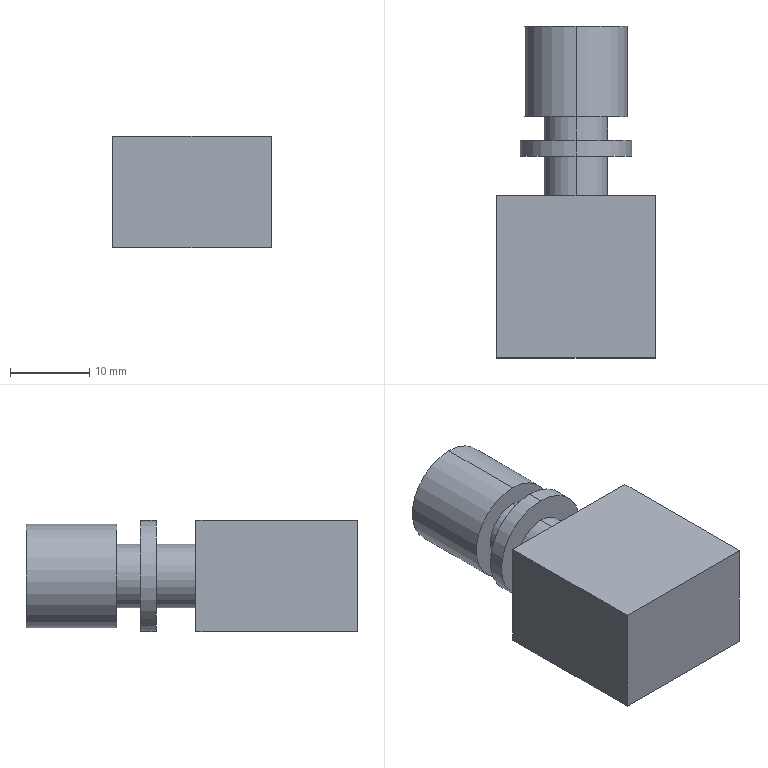Part | STEP file | A2A-4B | 1 solid | 18 faces | box 20 x 41.8 x 14 mm | volume 7935 mm3 | plane 10 | cylinder 8 | commonest cylinder face diameters 8 x4 13 x2 14 x2
STEP:
#1=CARTESIAN_POINT('',(0.,0.,0.));
#2=DIRECTION('',(0.,0.,1.));
#3=DIRECTION('',(1.,0.,0.));
#4=AXIS2_PLACEMENT_3D('',#1,#2,#3);
#5=CARTESIAN_POINT('',(0.,20.4,-4.));
#6=VERTEX_POINT('',#5);
#7=CARTESIAN_POINT('',(0.,20.4,4.));
#8=VERTEX_POINT('',#7);
#9=CARTESIAN_POINT('',(0.,20.4,0.));
#10=DIRECTION('',(0.,-1.,0.));
#11=DIRECTION('',(0.,0.,1.));
#12=AXIS2_PLACEMENT_3D('',#9,#10,#11);
#13=CIRCLE('',#12,4.);
#14=CARTESIAN_POINT('',(0.,41.8,0.));
#15=DIRECTION('',(0.,1.,0.));
#16=DIRECTION('',(0.,0.,1.));
#17=AXIS2_PLACEMENT_3D('',#14,#15,#16);
#18=CYLINDRICAL_SURFACE('',#17,4.);
#19=CARTESIAN_POINT('',(6.283,-21.4));
#20=DIRECTION('',(-1.,0.));
#21=VECTOR('',#20,1.);
#22=LINE('',#19,#21);
#23=(GEOMETRIC_REPRESENTATION_CONTEXT(2)PARAMETRIC_REPRESENTATION_CONTEXT()REPRESENTATION_CONTEXT('',''));
#24=DEFINITIONAL_REPRESENTATION('',(#22),#23);
#25=PCURVE('',#18,#24);
#26=CARTESIAN_POINT('',(10.,20.4,7.));
#27=DIRECTION('',(0.,1.,0.));
#28=DIRECTION('',(0.,0.,1.));
#29=AXIS2_PLACEMENT_3D('',#26,#27,#28);
#30=PLANE('',#29);
#31=CARTESIAN_POINT('',(-3.,-10.));
#32=CARTESIAN_POINT('',(-3.,-16.928));
#33=CARTESIAN_POINT('',(-9.,-13.464));
#34=CARTESIAN_POINT('',(-15.,-10.));
#35=CARTESIAN_POINT('',(-9.,-6.536));
#36=CARTESIAN_POINT('',(-3.,-3.072));
#37=CARTESIAN_POINT('',(-3.,-10.));
#38=(BOUNDED_CURVE()B_SPLINE_CURVE(2,(#31,#32,#33,#34,#35,#36,#37),.UNSPECIFIED.,.T.,.F.)B_SPLINE_CURVE_WITH_KNOTS((1,2,2,2,2,1),(-2.094,0.,2.094,4.189,6.283,8.378),.UNSPECIFIED.)CURVE()GEOMETRIC_REPRESENTATION_ITEM()RATIONAL_B_SPLINE_CURVE((1.,0.5,1.,0.5,1.,0.5,1.))REPRESENTATION_ITEM(''));
#39=(GEOMETRIC_REPRESENTATION_CONTEXT(2)PARAMETRIC_REPRESENTATION_CONTEXT()REPRESENTATION_CONTEXT('',''));
#40=DEFINITIONAL_REPRESENTATION('',(#38),#39);
#41=PCURVE('',#30,#40);
#42=SURFACE_CURVE('',#13,(#25,#41),.PCURVE_S1.);
#43=EDGE_CURVE('',#6,#8,#42,.T.);
#44=ORIENTED_EDGE('',*,*,#43,.F.);
#45=CARTESIAN_POINT('',(0.,25.4,-4.));
#46=VERTEX_POINT('',#45);
#47=CARTESIAN_POINT('',(0.,41.8,-4.));
#48=DIRECTION('',(0.,1.,0.));
#49=VECTOR('',#48,1.);
#50=LINE('',#47,#49);
#51=CARTESIAN_POINT('',(3.142,0.));
#52=DIRECTION('',(0.,1.));
#53=VECTOR('',#52,1.);
#54=LINE('',#51,#53);
#55=(GEOMETRIC_REPRESENTATION_CONTEXT(2)PARAMETRIC_REPRESENTATION_CONTEXT()REPRESENTATION_CONTEXT('',''));
#56=DEFINITIONAL_REPRESENTATION('',(#54),#55);
#57=PCURVE('',#18,#56);
#58=CARTESIAN_POINT('',(0.,41.8,0.));
#59=DIRECTION('',(0.,1.,0.));
#60=DIRECTION('',(0.,0.,1.));
#61=AXIS2_PLACEMENT_3D('',#58,#59,#60);
#62=CYLINDRICAL_SURFACE('',#61,4.);
#63=CARTESIAN_POINT('',(3.142,0.));
#64=DIRECTION('',(0.,1.));
#65=VECTOR('',#64,1.);
#66=LINE('',#63,#65);
#67=(GEOMETRIC_REPRESENTATION_CONTEXT(2)PARAMETRIC_REPRESENTATION_CONTEXT()REPRESENTATION_CONTEXT('',''));
#68=DEFINITIONAL_REPRESENTATION('',(#66),#67);
#69=PCURVE('',#62,#68);
#70=SURFACE_CURVE('',#50,(#57,#69),.PCURVE_S1.);
#71=EDGE_CURVE('',#6,#46,#70,.T.);
#72=ORIENTED_EDGE('',*,*,#71,.T.);
#73=CARTESIAN_POINT('',(0.,25.4,4.));
#74=VERTEX_POINT('',#73);
#75=CARTESIAN_POINT('',(0.,25.4,0.));
#76=DIRECTION('',(0.,-1.,0.));
#77=DIRECTION('',(0.,0.,1.));
#78=AXIS2_PLACEMENT_3D('',#75,#76,#77);
#79=CIRCLE('',#78,4.);
#80=CARTESIAN_POINT('',(6.283,-16.4));
#81=DIRECTION('',(-1.,0.));
#82=VECTOR('',#81,1.);
#83=LINE('',#80,#82);
#84=(GEOMETRIC_REPRESENTATION_CONTEXT(2)PARAMETRIC_REPRESENTATION_CONTEXT()REPRESENTATION_CONTEXT('',''));
#85=DEFINITIONAL_REPRESENTATION('',(#83),#84);
#86=PCURVE('',#18,#85);
#87=CARTESIAN_POINT('',(0.,25.4,4.));
#88=DIRECTION('',(0.,-1.,0.));
#89=DIRECTION('',(0.,0.,-1.));
#90=AXIS2_PLACEMENT_3D('',#87,#88,#89);
#91=PLANE('',#90);
#92=CARTESIAN_POINT('',(4.,0.));
#93=DIRECTION('',(-1.,0.));
#94=AXIS2_PLACEMENT_2D('',#92,#93);
#95=CIRCLE('',#94,4.);
#96=(GEOMETRIC_REPRESENTATION_CONTEXT(2)PARAMETRIC_REPRESENTATION_CONTEXT()REPRESENTATION_CONTEXT('',''));
#97=DEFINITIONAL_REPRESENTATION('',(#95),#96);
#98=PCURVE('',#91,#97);
#99=SURFACE_CURVE('',#79,(#86,#98),.PCURVE_S1.);
#100=EDGE_CURVE('',#46,#74,#99,.T.);
#101=ORIENTED_EDGE('',*,*,#100,.T.);
#102=CARTESIAN_POINT('',(0.,41.8,4.));
#103=DIRECTION('',(0.,1.,0.));
#104=VECTOR('',#103,1.);
#105=LINE('',#102,#104);
#106=CARTESIAN_POINT('',(0.,0.));
#107=DIRECTION('',(0.,1.));
#108=VECTOR('',#107,1.);
#109=LINE('',#106,#108);
#110=(GEOMETRIC_REPRESENTATION_CONTEXT(2)PARAMETRIC_REPRESENTATION_CONTEXT()REPRESENTATION_CONTEXT('',''));
#111=DEFINITIONAL_REPRESENTATION('',(#109),#110);
#112=PCURVE('',#18,#111);
#113=CARTESIAN_POINT('',(6.283,0.));
#114=DIRECTION('',(0.,1.));
#115=VECTOR('',#114,1.);
#116=LINE('',#113,#115);
#117=(GEOMETRIC_REPRESENTATION_CONTEXT(2)PARAMETRIC_REPRESENTATION_CONTEXT()REPRESENTATION_CONTEXT('',''));
#118=DEFINITIONAL_REPRESENTATION('',(#116),#117);
#119=PCURVE('',#62,#118);
#120=SURFACE_CURVE('',#105,(#112,#119),.PCURVE_S1.);
#121=EDGE_CURVE('',#8,#74,#120,.T.);
#122=ORIENTED_EDGE('',*,*,#121,.F.);
#123=EDGE_LOOP('',(#44,#72,#101,#122));
#124=FACE_BOUND('',#123,.T.);
#125=ADVANCED_FACE('',(#124),#18,.T.);
#126=CARTESIAN_POINT('',(0.,25.4,-7.));
#127=VERTEX_POINT('',#126);
#128=CARTESIAN_POINT('',(0.,25.4,7.));
#129=VERTEX_POINT('',#128);
#130=CARTESIAN_POINT('',(0.,25.4,0.));
#131=DIRECTION('',(0.,-1.,0.));
#132=DIRECTION('',(0.,0.,1.));
#133=AXIS2_PLACEMENT_3D('',#130,#131,#132);
#134=CIRCLE('',#133,7.);
#135=CARTESIAN_POINT('',(0.,41.8,0.));
#136=DIRECTION('',(0.,1.,0.));
#137=DIRECTION('',(0.,0.,1.));
#138=AXIS2_PLACEMENT_3D('',#135,#136,#137);
#139=CYLINDRICAL_SURFACE('',#138,7.);
#140=CARTESIAN_POINT('',(6.283,-16.4));
#141=DIRECTION('',(-1.,0.));
#142=VECTOR('',#141,1.);
#143=LINE('',#140,#142);
#144=(GEOMETRIC_REPRESENTATION_CONTEXT(2)PARAMETRIC_REPRESENTATION_CONTEXT()REPRESENTATION_CONTEXT('',''));
#145=DEFINITIONAL_REPRESENTATION('',(#143),#144);
#146=PCURVE('',#139,#145);
#147=CARTESIAN_POINT('',(4.,0.));
#148=DIRECTION('',(-1.,0.));
#149=AXIS2_PLACEMENT_2D('',#147,#148);
#150=CIRCLE('',#149,7.);
#151=(GEOMETRIC_REPRESENTATION_CONTEXT(2)PARAMETRIC_REPRESENTATION_CONTEXT()REPRESENTATION_CONTEXT('',''));
#152=DEFINITIONAL_REPRESENTATION('',(#150),#151);
#153=PCURVE('',#91,#152);
#154=SURFACE_CURVE('',#134,(#146,#153),.PCURVE_S1.);
#155=EDGE_CURVE('',#127,#129,#154,.T.);
#156=ORIENTED_EDGE('',*,*,#155,.F.);
#157=CARTESIAN_POINT('',(0.,27.4,-7.));
#158=VERTEX_POINT('',#157);
#159=CARTESIAN_POINT('',(0.,41.8,-7.));
#160=DIRECTION('',(0.,1.,0.));
#161=VECTOR('',#160,1.);
#162=LINE('',#159,#161);
#163=CARTESIAN_POINT('',(3.142,0.));
#164=DIRECTION('',(0.,1.));
#165=VECTOR('',#164,1.);
#166=LINE('',#163,#165);
#167=(GEOMETRIC_REPRESENTATION_CONTEXT(2)PARAMETRIC_REPRESENTATION_CONTEXT()REPRESENTATION_CONTEXT('',''));
#168=DEFINITIONAL_REPRESENTATION('',(#166),#167);
#169=PCURVE('',#139,#168);
#170=CARTESIAN_POINT('',(0.,41.8,0.));
#171=DIRECTION('',(0.,1.,0.));
#172=DIRECTION('',(0.,0.,1.));
#173=AXIS2_PLACEMENT_3D('',#170,#171,#172);
#174=CYLINDRICAL_SURFACE('',#173,7.);
#175=CARTESIAN_POINT('',(3.142,0.));
#176=DIRECTION('',(0.,1.));
#177=VECTOR('',#176,1.);
#178=LINE('',#175,#177);
#179=(GEOMETRIC_REPRESENTATION_CONTEXT(2)PARAMETRIC_REPRESENTATION_CONTEXT()REPRESENTATION_CONTEXT('',''));
#180=DEFINITIONAL_REPRESENTATION('',(#178),#179);
#181=PCURVE('',#174,#180);
#182=SURFACE_CURVE('',#162,(#169,#181),.PCURVE_S1.);
#183=EDGE_CURVE('',#127,#158,#182,.T.);
#184=ORIENTED_EDGE('',*,*,#183,.T.);
#185=CARTESIAN_POINT('',(0.,27.4,7.));
#186=VERTEX_POINT('',#185);
#187=CARTESIAN_POINT('',(0.,27.4,0.));
#188=DIRECTION('',(0.,-1.,0.));
#189=DIRECTION('',(0.,0.,1.));
#190=AXIS2_PLACEMENT_3D('',#187,#188,#189);
#191=CIRCLE('',#190,7.);
#192=CARTESIAN_POINT('',(6.283,-14.4));
#193=DIRECTION('',(-1.,0.));
#194=VECTOR('',#193,1.);
#195=LINE('',#192,#194);
#196=(GEOMETRIC_REPRESENTATION_CONTEXT(2)PARAMETRIC_REPRESENTATION_CONTEXT()REPRESENTATION_CONTEXT('',''));
#197=DEFINITIONAL_REPRESENTATION('',(#195),#196);
#198=PCURVE('',#139,#197);
#199=CARTESIAN_POINT('',(0.,27.4,7.));
#200=DIRECTION('',(0.,1.,0.));
#201=DIRECTION('',(0.,0.,1.));
#202=AXIS2_PLACEMENT_3D('',#199,#200,#201);
#203=PLANE('',#202);
#204=CARTESIAN_POINT('',(0.,0.));
#205=CARTESIAN_POINT('',(0.,-12.124));
#206=CARTESIAN_POINT('',(-10.5,-6.062));
#207=CARTESIAN_POINT('',(-21.,0.));
#208=CARTESIAN_POINT('',(-10.5,6.062));
#209=CARTESIAN_POINT('',(0.,12.124));
#210=CARTESIAN_POINT('',(0.,0.));
#211=(BOUNDED_CURVE()B_SPLINE_CURVE(2,(#204,#205,#206,#207,#208,#209,#210),.UNSPECIFIED.,.T.,.F.)B_SPLINE_CURVE_WITH_KNOTS((1,2,2,2,2,1),(-2.094,0.,2.094,4.189,6.283,8.378),.UNSPECIFIED.)CURVE()GEOMETRIC_REPRESENTATION_ITEM()RATIONAL_B_SPLINE_CURVE((1.,0.5,1.,0.5,1.,0.5,1.))REPRESENTATION_ITEM(''));
#212=(GEOMETRIC_REPRESENTATION_CONTEXT(2)PARAMETRIC_REPRESENTATION_CONTEXT()REPRESENTATION_CONTEXT('',''));
#213=DEFINITIONAL_REPRESENTATION('',(#211),#212);
#214=PCURVE('',#203,#213);
#215=SURFACE_CURVE('',#191,(#198,#214),.PCURVE_S1.);
#216=EDGE_CURVE('',#158,#186,#215,.T.);
#217=ORIENTED_EDGE('',*,*,#216,.T.);
#218=CARTESIAN_POINT('',(0.,41.8,7.));
#219=DIRECTION('',(0.,1.,0.));
#220=VECTOR('',#219,1.);
#221=LINE('',#218,#220);
#222=CARTESIAN_POINT('',(0.,0.));
#223=DIRECTION('',(0.,1.));
#224=VECTOR('',#223,1.);
#225=LINE('',#222,#224);
#226=(GEOMETRIC_REPRESENTATION_CONTEXT(2)PARAMETRIC_REPRESENTATION_CONTEXT()REPRESENTATION_CONTEXT('',''));
#227=DEFINITIONAL_REPRESENTATION('',(#225),#226);
#228=PCURVE('',#139,#227);
#229=CARTESIAN_POINT('',(6.283,0.));
#230=DIRECTION('',(0.,1.));
#231=VECTOR('',#230,1.);
#232=LINE('',#229,#231);
#233=(GEOMETRIC_REPRESENTATION_CONTEXT(2)PARAMETRIC_REPRESENTATION_CONTEXT()REPRESENTATION_CONTEXT('',''));
#234=DEFINITIONAL_REPRESENTATION('',(#232),#233);
#235=PCURVE('',#174,#234);
#236=SURFACE_CURVE('',#221,(#228,#235),.PCURVE_S1.);
#237=EDGE_CURVE('',#129,#186,#236,.T.);
#238=ORIENTED_EDGE('',*,*,#237,.F.);
#239=EDGE_LOOP('',(#156,#184,#217,#238));
#240=FACE_BOUND('',#239,.T.);
#241=ADVANCED_FACE('',(#240),#139,.T.);
#242=CARTESIAN_POINT('',(0.,27.4,-4.));
#243=VERTEX_POINT('',#242);
#244=CARTESIAN_POINT('',(0.,27.4,4.));
#245=VERTEX_POINT('',#244);
#246=CARTESIAN_POINT('',(0.,27.4,0.));
#247=DIRECTION('',(0.,-1.,0.));
#248=DIRECTION('',(0.,0.,1.));
#249=AXIS2_PLACEMENT_3D('',#246,#247,#248);
#250=CIRCLE('',#249,4.);
#251=CARTESIAN_POINT('',(0.,41.8,0.));
#252=DIRECTION('',(0.,1.,0.));
#253=DIRECTION('',(0.,0.,1.));
#254=AXIS2_PLACEMENT_3D('',#251,#252,#253);
#255=CYLINDRICAL_SURFACE('',#254,4.);
#256=CARTESIAN_POINT('',(6.283,-14.4));
#257=DIRECTION('',(-1.,0.));
#258=VECTOR('',#257,1.);
#259=LINE('',#256,#258);
#260=(GEOMETRIC_REPRESENTATION_CONTEXT(2)PARAMETRIC_REPRESENTATION_CONTEXT()REPRESENTATION_CONTEXT('',''));
#261=DEFINITIONAL_REPRESENTATION('',(#259),#260);
#262=PCURVE('',#255,#261);
#263=CARTESIAN_POINT('',(-3.,0.));
#264=CARTESIAN_POINT('',(-3.,-6.928));
#265=CARTESIAN_POINT('',(-9.,-3.464));
#266=CARTESIAN_POINT('',(-15.,0.));
#267=CARTESIAN_POINT('',(-9.,3.464));
#268=CARTESIAN_POINT('',(-3.,6.928));
#269=CARTESIAN_POINT('',(-3.,0.));
#270=(BOUNDED_CURVE()B_SPLINE_CURVE(2,(#263,#264,#265,#266,#267,#268,#269),.UNSPECIFIED.,.T.,.F.)B_SPLINE_CURVE_WITH_KNOTS((1,2,2,2,2,1),(-2.094,0.,2.094,4.189,6.283,8.378),.UNSPECIFIED.)CURVE()GEOMETRIC_REPRESENTATION_ITEM()RATIONAL_B_SPLINE_CURVE((1.,0.5,1.,0.5,1.,0.5,1.))REPRESENTATION_ITEM(''));
#271=(GEOMETRIC_REPRESENTATION_CONTEXT(2)PARAMETRIC_REPRESENTATION_CONTEXT()REPRESENTATION_CONTEXT('',''));
#272=DEFINITIONAL_REPRESENTATION('',(#270),#271);
#273=PCURVE('',#203,#272);
#274=SURFACE_CURVE('',#250,(#262,#273),.PCURVE_S1.);
#275=EDGE_CURVE('',#243,#245,#274,.T.);
#276=ORIENTED_EDGE('',*,*,#275,.F.);
#277=CARTESIAN_POINT('',(0.,30.4,-4.));
#278=VERTEX_POINT('',#277);
#279=CARTESIAN_POINT('',(0.,41.8,-4.));
#280=DIRECTION('',(0.,1.,0.));
#281=VECTOR('',#280,1.);
#282=LINE('',#279,#281);
#283=CARTESIAN_POINT('',(3.142,0.));
#284=DIRECTION('',(0.,1.));
#285=VECTOR('',#284,1.);
#286=LINE('',#283,#285);
#287=(GEOMETRIC_REPRESENTATION_CONTEXT(2)PARAMETRIC_REPRESENTATION_CONTEXT()REPRESENTATION_CONTEXT('',''));
#288=DEFINITIONAL_REPRESENTATION('',(#286),#287);
#289=PCURVE('',#255,#288);
#290=CARTESIAN_POINT('',(0.,41.8,0.));
#291=DIRECTION('',(0.,1.,0.));
#292=DIRECTION('',(0.,0.,1.));
#293=AXIS2_PLACEMENT_3D('',#290,#291,#292);
#294=CYLINDRICAL_SURFACE('',#293,4.);
#295=CARTESIAN_POINT('',(3.142,0.));
#296=DIRECTION('',(0.,1.));
#297=VECTOR('',#296,1.);
#298=LINE('',#295,#297);
#299=(GEOMETRIC_REPRESENTATION_CONTEXT(2)PARAMETRIC_REPRESENTATION_CONTEXT()REPRESENTATION_CONTEXT('',''));
#300=DEFINITIONAL_REPRESENTATION('',(#298),#299);
#301=PCURVE('',#294,#300);
#302=SURFACE_CURVE('',#282,(#289,#301),.PCURVE_S1.);
#303=EDGE_CURVE('',#243,#278,#302,.T.);
#304=ORIENTED_EDGE('',*,*,#303,.T.);
#305=CARTESIAN_POINT('',(0.,30.4,4.));
#306=VERTEX_POINT('',#305);
#307=CARTESIAN_POINT('',(0.,30.4,0.));
#308=DIRECTION('',(0.,-1.,0.));
#309=DIRECTION('',(0.,0.,1.));
#310=AXIS2_PLACEMENT_3D('',#307,#308,#309);
#311=CIRCLE('',#310,4.);
#312=CARTESIAN_POINT('',(6.283,-11.4));
#313=DIRECTION('',(-1.,0.));
#314=VECTOR('',#313,1.);
#315=LINE('',#312,#314);
#316=(GEOMETRIC_REPRESENTATION_CONTEXT(2)PARAMETRIC_REPRESENTATION_CONTEXT()REPRESENTATION_CONTEXT('',''));
#317=DEFINITIONAL_REPRESENTATION('',(#315),#316);
#318=PCURVE('',#255,#317);
#319=CARTESIAN_POINT('',(0.,30.4,6.5));
#320=DIRECTION('',(0.,-1.,0.));
#321=DIRECTION('',(0.,0.,-1.));
#322=AXIS2_PLACEMENT_3D('',#319,#320,#321);
#323=PLANE('',#322);
#324=CARTESIAN_POINT('',(6.5,0.));
#325=DIRECTION('',(-1.,0.));
#326=AXIS2_PLACEMENT_2D('',#324,#325);
#327=CIRCLE('',#326,4.);
#328=(GEOMETRIC_REPRESENTATION_CONTEXT(2)PARAMETRIC_REPRESENTATION_CONTEXT()REPRESENTATION_CONTEXT('',''));
#329=DEFINITIONAL_REPRESENTATION('',(#327),#328);
#330=PCURVE('',#323,#329);
#331=SURFACE_CURVE('',#311,(#318,#330),.PCURVE_S1.);
#332=EDGE_CURVE('',#278,#306,#331,.T.);
#333=ORIENTED_EDGE('',*,*,#332,.T.);
#334=CARTESIAN_POINT('',(0.,41.8,4.));
#335=DIRECTION('',(0.,1.,0.));
#336=VECTOR('',#335,1.);
#337=LINE('',#334,#336);
#338=CARTESIAN_POINT('',(0.,0.));
#339=DIRECTION('',(0.,1.));
#340=VECTOR('',#339,1.);
#341=LINE('',#338,#340);
#342=(GEOMETRIC_REPRESENTATION_CONTEXT(2)PARAMETRIC_REPRESENTATION_CONTEXT()REPRESENTATION_CONTEXT('',''));
#343=DEFINITIONAL_REPRESENTATION('',(#341),#342);
#344=PCURVE('',#255,#343);
#345=CARTESIAN_POINT('',(6.283,0.));
#346=DIRECTION('',(0.,1.));
#347=VECTOR('',#346,1.);
#348=LINE('',#345,#347);
#349=(GEOMETRIC_REPRESENTATION_CONTEXT(2)PARAMETRIC_REPRESENTATION_CONTEXT()REPRESENTATION_CONTEXT('',''));
#350=DEFINITIONAL_REPRESENTATION('',(#348),#349);
#351=PCURVE('',#294,#350);
#352=SURFACE_CURVE('',#337,(#344,#351),.PCURVE_S1.);
#353=EDGE_CURVE('',#245,#306,#352,.T.);
#354=ORIENTED_EDGE('',*,*,#353,.F.);
#355=EDGE_LOOP('',(#276,#304,#333,#354));
#356=FACE_BOUND('',#355,.T.);
#357=ADVANCED_FACE('',(#356),#255,.T.);
#358=CARTESIAN_POINT('',(0.,30.4,-6.5));
#359=VERTEX_POINT('',#358);
#360=CARTESIAN_POINT('',(0.,30.4,6.5));
#361=VERTEX_POINT('',#360);
#362=CARTESIAN_POINT('',(0.,30.4,0.));
#363=DIRECTION('',(0.,-1.,0.));
#364=DIRECTION('',(0.,0.,1.));
#365=AXIS2_PLACEMENT_3D('',#362,#363,#364);
#366=CIRCLE('',#365,6.5);
#367=CARTESIAN_POINT('',(0.,41.8,0.));
#368=DIRECTION('',(0.,1.,0.));
#369=DIRECTION('',(0.,0.,1.));
#370=AXIS2_PLACEMENT_3D('',#367,#368,#369);
#371=CYLINDRICAL_SURFACE('',#370,6.5);
#372=CARTESIAN_POINT('',(6.283,-11.4));
#373=DIRECTION('',(-1.,0.));
#374=VECTOR('',#373,1.);
#375=LINE('',#372,#374);
#376=(GEOMETRIC_REPRESENTATION_CONTEXT(2)PARAMETRIC_REPRESENTATION_CONTEXT()REPRESENTATION_CONTEXT('',''));
#377=DEFINITIONAL_REPRESENTATION('',(#375),#376);
#378=PCURVE('',#371,#377);
#379=CARTESIAN_POINT('',(6.5,0.));
#380=DIRECTION('',(-1.,0.));
#381=AXIS2_PLACEMENT_2D('',#379,#380);
#382=CIRCLE('',#381,6.5);
#383=(GEOMETRIC_REPRESENTATION_CONTEXT(2)PARAMETRIC_REPRESENTATION_CONTEXT()REPRESENTATION_CONTEXT('',''));
#384=DEFINITIONAL_REPRESENTATION('',(#382),#383);
#385=PCURVE('',#323,#384);
#386=SURFACE_CURVE('',#366,(#378,#385),.PCURVE_S1.);
#387=EDGE_CURVE('',#359,#361,#386,.T.);
#388=ORIENTED_EDGE('',*,*,#387,.F.);
#389=CARTESIAN_POINT('',(0.,41.8,-6.5));
#390=VERTEX_POINT('',#389);
#391=CARTESIAN_POINT('',(0.,41.8,-6.5));
#392=DIRECTION('',(0.,1.,0.));
#393=VECTOR('',#392,1.);
#394=LINE('',#391,#393);
#395=CARTESIAN_POINT('',(3.142,0.));
#396=DIRECTION('',(0.,1.));
#397=VECTOR('',#396,1.);
#398=LINE('',#395,#397);
#399=(GEOMETRIC_REPRESENTATION_CONTEXT(2)PARAMETRIC_REPRESENTATION_CONTEXT()REPRESENTATION_CONTEXT('',''));
#400=DEFINITIONAL_REPRESENTATION('',(#398),#399);
#401=PCURVE('',#371,#400);
#402=CARTESIAN_POINT('',(0.,41.8,0.));
#403=DIRECTION('',(0.,1.,0.));
#404=DIRECTION('',(0.,0.,1.));
#405=AXIS2_PLACEMENT_3D('',#402,#403,#404);
#406=CYLINDRICAL_SURFACE('',#405,6.5);
#407=CARTESIAN_POINT('',(3.142,0.));
#408=DIRECTION('',(0.,1.));
#409=VECTOR('',#408,1.);
#410=LINE('',#407,#409);
#411=(GEOMETRIC_REPRESENTATION_CONTEXT(2)PARAMETRIC_REPRESENTATION_CONTEXT()REPRESENTATION_CONTEXT('',''));
#412=DEFINITIONAL_REPRESENTATION('',(#410),#411);
#413=PCURVE('',#406,#412);
#414=SURFACE_CURVE('',#394,(#401,#413),.PCURVE_S1.);
#415=EDGE_CURVE('',#359,#390,#414,.T.);
#416=ORIENTED_EDGE('',*,*,#415,.T.);
#417=CARTESIAN_POINT('',(0.,41.8,6.5));
#418=VERTEX_POINT('',#417);
#419=CARTESIAN_POINT('',(0.,41.8,0.));
#420=DIRECTION('',(0.,-1.,0.));
#421=DIRECTION('',(0.,0.,1.));
#422=AXIS2_PLACEMENT_3D('',#419,#420,#421);
#423=CIRCLE('',#422,6.5);
#424=CARTESIAN_POINT('',(6.283,0.));
#425=DIRECTION('',(-1.,0.));
#426=VECTOR('',#425,1.);
#427=LINE('',#424,#426);
#428=(GEOMETRIC_REPRESENTATION_CONTEXT(2)PARAMETRIC_REPRESENTATION_CONTEXT()REPRESENTATION_CONTEXT('',''));
#429=DEFINITIONAL_REPRESENTATION('',(#427),#428);
#430=PCURVE('',#371,#429);
#431=CARTESIAN_POINT('',(0.,41.8,6.5));
#432=DIRECTION('',(0.,1.,0.));
#433=DIRECTION('',(0.,0.,1.));
#434=AXIS2_PLACEMENT_3D('',#431,#432,#433);
#435=PLANE('',#434);
#436=CARTESIAN_POINT('',(0.,0.));
#437=CARTESIAN_POINT('',(0.,-11.258));
#438=CARTESIAN_POINT('',(-9.75,-5.629));
#439=CARTESIAN_POINT('',(-19.5,0.));
#440=CARTESIAN_POINT('',(-9.75,5.629));
#441=CARTESIAN_POINT('',(0.,11.258));
#442=CARTESIAN_POINT('',(0.,0.));
#443=(BOUNDED_CURVE()B_SPLINE_CURVE(2,(#436,#437,#438,#439,#440,#441,#442),.UNSPECIFIED.,.T.,.F.)B_SPLINE_CURVE_WITH_KNOTS((1,2,2,2,2,1),(-2.094,0.,2.094,4.189,6.283,8.378),.UNSPECIFIED.)CURVE()GEOMETRIC_REPRESENTATION_ITEM()RATIONAL_B_SPLINE_CURVE((1.,0.5,1.,0.5,1.,0.5,1.))REPRESENTATION_ITEM(''));
#444=(GEOMETRIC_REPRESENTATION_CONTEXT(2)PARAMETRIC_REPRESENTATION_CONTEXT()REPRESENTATION_CONTEXT('',''));
#445=DEFINITIONAL_REPRESENTATION('',(#443),#444);
#446=PCURVE('',#435,#445);
#447=SURFACE_CURVE('',#423,(#430,#446),.PCURVE_S1.);
#448=EDGE_CURVE('',#390,#418,#447,.T.);
#449=ORIENTED_EDGE('',*,*,#448,.T.);
#450=CARTESIAN_POINT('',(0.,41.8,6.5));
#451=DIRECTION('',(0.,1.,0.));
#452=VECTOR('',#451,1.);
#453=LINE('',#450,#452);
#454=CARTESIAN_POINT('',(0.,0.));
#455=DIRECTION('',(0.,1.));
#456=VECTOR('',#455,1.);
#457=LINE('',#454,#456);
#458=(GEOMETRIC_REPRESENTATION_CONTEXT(2)PARAMETRIC_REPRESENTATION_CONTEXT()REPRESENTATION_CONTEXT('',''));
#459=DEFINITIONAL_REPRESENTATION('',(#457),#458);
#460=PCURVE('',#371,#459);
#461=CARTESIAN_POINT('',(6.283,0.));
#462=DIRECTION('',(0.,1.));
#463=VECTOR('',#462,1.);
#464=LINE('',#461,#463);
#465=(GEOMETRIC_REPRESENTATION_CONTEXT(2)PARAMETRIC_REPRESENTATION_CONTEXT()REPRESENTATION_CONTEXT('',''));
#466=DEFINITIONAL_REPRESENTATION('',(#464),#465);
#467=PCURVE('',#406,#466);
#468=SURFACE_CURVE('',#453,(#460,#467),.PCURVE_S1.);
#469=EDGE_CURVE('',#361,#418,#468,.T.);
#470=ORIENTED_EDGE('',*,*,#469,.F.);
#471=EDGE_LOOP('',(#388,#416,#449,#470));
#472=FACE_BOUND('',#471,.T.);
#473=ADVANCED_FACE('',(#472),#371,.T.);
#474=CARTESIAN_POINT('',(-10.,20.4,-7.));
#475=VERTEX_POINT('',#474);
#476=CARTESIAN_POINT('',(-10.,0.,-7.));
#477=VERTEX_POINT('',#476);
#478=CARTESIAN_POINT('',(-10.,20.4,-7.));
#479=DIRECTION('',(0.,-1.,0.));
#480=VECTOR('',#479,1.);
#481=LINE('',#478,#480);
#482=CARTESIAN_POINT('',(-10.,20.4,-7.));
#483=DIRECTION('',(0.,0.,1.));
#484=DIRECTION('',(1.,0.,0.));
#485=AXIS2_PLACEMENT_3D('',#482,#483,#484);
#486=PLANE('',#485);
#487=CARTESIAN_POINT('',(0.,0.));
#488=DIRECTION('',(0.,-1.));
#489=VECTOR('',#488,1.);
#490=LINE('',#487,#489);
#491=(GEOMETRIC_REPRESENTATION_CONTEXT(2)PARAMETRIC_REPRESENTATION_CONTEXT()REPRESENTATION_CONTEXT('',''));
#492=DEFINITIONAL_REPRESENTATION('',(#490),#491);
#493=PCURVE('',#486,#492);
#494=CARTESIAN_POINT('',(-10.,20.4,-7.));
#495=DIRECTION('',(1.,0.,0.));
#496=DIRECTION('',(0.,0.,-1.));
#497=AXIS2_PLACEMENT_3D('',#494,#495,#496);
#498=PLANE('',#497);
#499=CARTESIAN_POINT('',(0.,0.));
#500=DIRECTION('',(0.,-1.));
#501=VECTOR('',#500,1.);
#502=LINE('',#499,#501);
#503=(GEOMETRIC_REPRESENTATION_CONTEXT(2)PARAMETRIC_REPRESENTATION_CONTEXT()REPRESENTATION_CONTEXT('',''));
#504=DEFINITIONAL_REPRESENTATION('',(#502),#503);
#505=PCURVE('',#498,#504);
#506=SURFACE_CURVE('',#481,(#493,#505),.PCURVE_S1.);
#507=EDGE_CURVE('',#475,#477,#506,.T.);
#508=ORIENTED_EDGE('',*,*,#507,.F.);
#509=CARTESIAN_POINT('',(10.,20.4,-7.));
#510=VERTEX_POINT('',#509);
#511=CARTESIAN_POINT('',(-10.,20.4,-7.));
#512=DIRECTION('',(-1.,0.,0.));
#513=VECTOR('',#512,1.);
#514=LINE('',#511,#513);
#515=CARTESIAN_POINT('',(0.,0.));
#516=DIRECTION('',(-1.,0.));
#517=VECTOR('',#516,1.);
#518=LINE('',#515,#517);
#519=(GEOMETRIC_REPRESENTATION_CONTEXT(2)PARAMETRIC_REPRESENTATION_CONTEXT()REPRESENTATION_CONTEXT('',''));
#520=DEFINITIONAL_REPRESENTATION('',(#518),#519);
#521=PCURVE('',#486,#520);
#522=CARTESIAN_POINT('',(-14.,-20.));
#523=DIRECTION('',(0.,-1.));
#524=VECTOR('',#523,1.);
#525=LINE('',#522,#524);
#526=(GEOMETRIC_REPRESENTATION_CONTEXT(2)PARAMETRIC_REPRESENTATION_CONTEXT()REPRESENTATION_CONTEXT('',''));
#527=DEFINITIONAL_REPRESENTATION('',(#525),#526);
#528=PCURVE('',#30,#527);
#529=SURFACE_CURVE('',#514,(#521,#528),.PCURVE_S1.);
#530=EDGE_CURVE('',#510,#475,#529,.T.);
#531=ORIENTED_EDGE('',*,*,#530,.F.);
#532=CARTESIAN_POINT('',(10.,0.,-7.));
#533=VERTEX_POINT('',#532);
#534=CARTESIAN_POINT('',(10.,20.4,-7.));
#535=DIRECTION('',(0.,1.,0.));
#536=VECTOR('',#535,1.);
#537=LINE('',#534,#536);
#538=CARTESIAN_POINT('',(20.,0.));
#539=DIRECTION('',(0.,1.));
#540=VECTOR('',#539,1.);
#541=LINE('',#538,#540);
#542=(GEOMETRIC_REPRESENTATION_CONTEXT(2)PARAMETRIC_REPRESENTATION_CONTEXT()REPRESENTATION_CONTEXT('',''));
#543=DEFINITIONAL_REPRESENTATION('',(#541),#542);
#544=PCURVE('',#486,#543);
#545=CARTESIAN_POINT('',(10.,20.4,-7.));
#546=DIRECTION('',(-1.,0.,0.));
#547=DIRECTION('',(0.,0.,1.));
#548=AXIS2_PLACEMENT_3D('',#545,#546,#547);
#549=PLANE('',#548);
#550=CARTESIAN_POINT('',(0.,0.));
#551=DIRECTION('',(0.,1.));
#552=VECTOR('',#551,1.);
#553=LINE('',#550,#552);
#554=(GEOMETRIC_REPRESENTATION_CONTEXT(2)PARAMETRIC_REPRESENTATION_CONTEXT()REPRESENTATION_CONTEXT('',''));
#555=DEFINITIONAL_REPRESENTATION('',(#553),#554);
#556=PCURVE('',#549,#555);
#557=SURFACE_CURVE('',#537,(#544,#556),.PCURVE_S1.);
#558=EDGE_CURVE('',#533,#510,#557,.T.);
#559=ORIENTED_EDGE('',*,*,#558,.F.);
#560=CARTESIAN_POINT('',(-10.,0.,-7.));
#561=DIRECTION('',(1.,0.,0.));
#562=VECTOR('',#561,1.);
#563=LINE('',#560,#562);
#564=CARTESIAN_POINT('',(0.,-20.4));
#565=DIRECTION('',(1.,0.));
#566=VECTOR('',#565,1.);
#567=LINE('',#564,#566);
#568=(GEOMETRIC_REPRESENTATION_CONTEXT(2)PARAMETRIC_REPRESENTATION_CONTEXT()REPRESENTATION_CONTEXT('',''));
#569=DEFINITIONAL_REPRESENTATION('',(#567),#568);
#570=PCURVE('',#486,#569);
#571=CARTESIAN_POINT('',(10.,0.,7.));
#572=DIRECTION('',(0.,1.,0.));
#573=DIRECTION('',(0.,0.,1.));
#574=AXIS2_PLACEMENT_3D('',#571,#572,#573);
#575=PLANE('',#574);
#576=CARTESIAN_POINT('',(-14.,-20.));
#577=DIRECTION('',(0.,1.));
#578=VECTOR('',#577,1.);
#579=LINE('',#576,#578);
#580=(GEOMETRIC_REPRESENTATION_CONTEXT(2)PARAMETRIC_REPRESENTATION_CONTEXT()REPRESENTATION_CONTEXT('',''));
#581=DEFINITIONAL_REPRESENTATION('',(#579),#580);
#582=PCURVE('',#575,#581);
#583=SURFACE_CURVE('',#563,(#570,#582),.PCURVE_S1.);
#584=EDGE_CURVE('',#477,#533,#583,.T.);
#585=ORIENTED_EDGE('',*,*,#584,.F.);
#586=EDGE_LOOP('',(#508,#531,#559,#585));
#587=FACE_BOUND('',#586,.T.);
#588=ADVANCED_FACE('',(#587),#486,.F.);
#589=CARTESIAN_POINT('',(-10.,0.,7.));
#590=VERTEX_POINT('',#589);
#591=CARTESIAN_POINT('',(10.,0.,7.));
#592=VERTEX_POINT('',#591);
#593=CARTESIAN_POINT('',(10.,0.,7.));
#594=DIRECTION('',(1.,0.,0.));
#595=VECTOR('',#594,1.);
#596=LINE('',#593,#595);
#597=CARTESIAN_POINT('',(0.,0.));
#598=DIRECTION('',(0.,1.));
#599=VECTOR('',#598,1.);
#600=LINE('',#597,#599);
#601=(GEOMETRIC_REPRESENTATION_CONTEXT(2)PARAMETRIC_REPRESENTATION_CONTEXT()REPRESENTATION_CONTEXT('',''));
#602=DEFINITIONAL_REPRESENTATION('',(#600),#601);
#603=PCURVE('',#575,#602);
#604=CARTESIAN_POINT('',(-10.,20.4,7.));
#605=DIRECTION('',(0.,0.,-1.));
#606=DIRECTION('',(-1.,0.,0.));
#607=AXIS2_PLACEMENT_3D('',#604,#605,#606);
#608=PLANE('',#607);
#609=CARTESIAN_POINT('',(-20.,-20.4));
#610=DIRECTION('',(-1.,0.));
#611=VECTOR('',#610,1.);
#612=LINE('',#609,#611);
#613=(GEOMETRIC_REPRESENTATION_CONTEXT(2)PARAMETRIC_REPRESENTATION_CONTEXT()REPRESENTATION_CONTEXT('',''));
#614=DEFINITIONAL_REPRESENTATION('',(#612),#613);
#615=PCURVE('',#608,#614);
#616=SURFACE_CURVE('',#596,(#603,#615),.PCURVE_S1.);
#617=EDGE_CURVE('',#590,#592,#616,.T.);
#618=ORIENTED_EDGE('',*,*,#617,.F.);
#619=CARTESIAN_POINT('',(-10.,0.,7.));
#620=DIRECTION('',(0.,0.,1.));
#621=VECTOR('',#620,1.);
#622=LINE('',#619,#621);
#623=CARTESIAN_POINT('',(0.,-20.));
#624=DIRECTION('',(1.,0.));
#625=VECTOR('',#624,1.);
#626=LINE('',#623,#625);
#627=(GEOMETRIC_REPRESENTATION_CONTEXT(2)PARAMETRIC_REPRESENTATION_CONTEXT()REPRESENTATION_CONTEXT('',''));
#628=DEFINITIONAL_REPRESENTATION('',(#626),#627);
#629=PCURVE('',#575,#628);
#630=CARTESIAN_POINT('',(-14.,-20.4));
#631=DIRECTION('',(-1.,0.));
#632=VECTOR('',#631,1.);
#633=LINE('',#630,#632);
#634=(GEOMETRIC_REPRESENTATION_CONTEXT(2)PARAMETRIC_REPRESENTATION_CONTEXT()REPRESENTATION_CONTEXT('',''));
#635=DEFINITIONAL_REPRESENTATION('',(#633),#634);
#636=PCURVE('',#498,#635);
#637=SURFACE_CURVE('',#622,(#629,#636),.PCURVE_S1.);
#638=EDGE_CURVE('',#477,#590,#637,.T.);
#639=ORIENTED_EDGE('',*,*,#638,.F.);
#640=ORIENTED_EDGE('',*,*,#584,.T.);
#641=CARTESIAN_POINT('',(10.,0.,7.));
#642=DIRECTION('',(0.,0.,-1.));
#643=VECTOR('',#642,1.);
#644=LINE('',#641,#643);
#645=CARTESIAN_POINT('',(0.,0.));
#646=DIRECTION('',(-1.,0.));
#647=VECTOR('',#646,1.);
#648=LINE('',#645,#647);
#649=(GEOMETRIC_REPRESENTATION_CONTEXT(2)PARAMETRIC_REPRESENTATION_CONTEXT()REPRESENTATION_CONTEXT('',''));
#650=DEFINITIONAL_REPRESENTATION('',(#648),#649);
#651=PCURVE('',#575,#650);
#652=CARTESIAN_POINT('',(14.,-20.4));
#653=DIRECTION('',(-1.,0.));
#654=VECTOR('',#653,1.);
#655=LINE('',#652,#654);
#656=(GEOMETRIC_REPRESENTATION_CONTEXT(2)PARAMETRIC_REPRESENTATION_CONTEXT()REPRESENTATION_CONTEXT('',''));
#657=DEFINITIONAL_REPRESENTATION('',(#655),#656);
#658=PCURVE('',#549,#657);
#659=SURFACE_CURVE('',#644,(#651,#658),.PCURVE_S1.);
#660=EDGE_CURVE('',#592,#533,#659,.T.);
#661=ORIENTED_EDGE('',*,*,#660,.F.);
#662=EDGE_LOOP('',(#618,#639,#640,#661));
#663=FACE_BOUND('',#662,.T.);
#664=ADVANCED_FACE('',(#663),#575,.F.);
#665=CARTESIAN_POINT('',(-10.,20.4,7.));
#666=VERTEX_POINT('',#665);
#667=CARTESIAN_POINT('',(-10.,20.4,7.));
#668=DIRECTION('',(0.,-1.,0.));
#669=VECTOR('',#668,1.);
#670=LINE('',#667,#669);
#671=CARTESIAN_POINT('',(-14.,0.));
#672=DIRECTION('',(0.,-1.));
#673=VECTOR('',#672,1.);
#674=LINE('',#671,#673);
#675=(GEOMETRIC_REPRESENTATION_CONTEXT(2)PARAMETRIC_REPRESENTATION_CONTEXT()REPRESENTATION_CONTEXT('',''));
#676=DEFINITIONAL_REPRESENTATION('',(#674),#675);
#677=PCURVE('',#498,#676);
#678=CARTESIAN_POINT('',(0.,0.));
#679=DIRECTION('',(0.,-1.));
#680=VECTOR('',#679,1.);
#681=LINE('',#678,#680);
#682=(GEOMETRIC_REPRESENTATION_CONTEXT(2)PARAMETRIC_REPRESENTATION_CONTEXT()REPRESENTATION_CONTEXT('',''));
#683=DEFINITIONAL_REPRESENTATION('',(#681),#682);
#684=PCURVE('',#608,#683);
#685=SURFACE_CURVE('',#670,(#677,#684),.PCURVE_S1.);
#686=EDGE_CURVE('',#666,#590,#685,.T.);
#687=ORIENTED_EDGE('',*,*,#686,.F.);
#688=CARTESIAN_POINT('',(-10.,20.4,-7.));
#689=DIRECTION('',(0.,0.,1.));
#690=VECTOR('',#689,1.);
#691=LINE('',#688,#690);
#692=CARTESIAN_POINT('',(0.,0.));
#693=DIRECTION('',(-1.,0.));
#694=VECTOR('',#693,1.);
#695=LINE('',#692,#694);
#696=(GEOMETRIC_REPRESENTATION_CONTEXT(2)PARAMETRIC_REPRESENTATION_CONTEXT()REPRESENTATION_CONTEXT('',''));
#697=DEFINITIONAL_REPRESENTATION('',(#695),#696);
#698=PCURVE('',#498,#697);
#699=CARTESIAN_POINT('',(-14.,-20.));
#700=DIRECTION('',(1.,0.));
#701=VECTOR('',#700,1.);
#702=LINE('',#699,#701);
#703=(GEOMETRIC_REPRESENTATION_CONTEXT(2)PARAMETRIC_REPRESENTATION_CONTEXT()REPRESENTATION_CONTEXT('',''));
#704=DEFINITIONAL_REPRESENTATION('',(#702),#703);
#705=PCURVE('',#30,#704);
#706=SURFACE_CURVE('',#691,(#698,#705),.PCURVE_S1.);
#707=EDGE_CURVE('',#475,#666,#706,.T.);
#708=ORIENTED_EDGE('',*,*,#707,.F.);
#709=ORIENTED_EDGE('',*,*,#507,.T.);
#710=ORIENTED_EDGE('',*,*,#638,.T.);
#711=EDGE_LOOP('',(#687,#708,#709,#710));
#712=FACE_BOUND('',#711,.T.);
#713=ADVANCED_FACE('',(#712),#498,.F.);
#714=ORIENTED_EDGE('',*,*,#707,.T.);
#715=CARTESIAN_POINT('',(10.,20.4,7.));
#716=VERTEX_POINT('',#715);
#717=CARTESIAN_POINT('',(10.,20.4,7.));
#718=DIRECTION('',(1.,0.,0.));
#719=VECTOR('',#718,1.);
#720=LINE('',#717,#719);
#721=CARTESIAN_POINT('',(0.,0.));
#722=DIRECTION('',(0.,1.));
#723=VECTOR('',#722,1.);
#724=LINE('',#721,#723);
#725=(GEOMETRIC_REPRESENTATION_CONTEXT(2)PARAMETRIC_REPRESENTATION_CONTEXT()REPRESENTATION_CONTEXT('',''));
#726=DEFINITIONAL_REPRESENTATION('',(#724),#725);
#727=PCURVE('',#30,#726);
#728=CARTESIAN_POINT('',(-20.,0.));
#729=DIRECTION('',(-1.,0.));
#730=VECTOR('',#729,1.);
#731=LINE('',#728,#730);
#732=(GEOMETRIC_REPRESENTATION_CONTEXT(2)PARAMETRIC_REPRESENTATION_CONTEXT()REPRESENTATION_CONTEXT('',''));
#733=DEFINITIONAL_REPRESENTATION('',(#731),#732);
#734=PCURVE('',#608,#733);
#735=SURFACE_CURVE('',#720,(#727,#734),.PCURVE_S1.);
#736=EDGE_CURVE('',#666,#716,#735,.T.);
#737=ORIENTED_EDGE('',*,*,#736,.T.);
#738=CARTESIAN_POINT('',(10.,20.4,7.));
#739=DIRECTION('',(0.,0.,-1.));
#740=VECTOR('',#739,1.);
#741=LINE('',#738,#740);
#742=CARTESIAN_POINT('',(0.,0.));
#743=DIRECTION('',(-1.,0.));
#744=VECTOR('',#743,1.);
#745=LINE('',#742,#744);
#746=(GEOMETRIC_REPRESENTATION_CONTEXT(2)PARAMETRIC_REPRESENTATION_CONTEXT()REPRESENTATION_CONTEXT('',''));
#747=DEFINITIONAL_REPRESENTATION('',(#745),#746);
#748=PCURVE('',#30,#747);
#749=CARTESIAN_POINT('',(14.,0.));
#750=DIRECTION('',(-1.,0.));
#751=VECTOR('',#750,1.);
#752=LINE('',#749,#751);
#753=(GEOMETRIC_REPRESENTATION_CONTEXT(2)PARAMETRIC_REPRESENTATION_CONTEXT()REPRESENTATION_CONTEXT('',''));
#754=DEFINITIONAL_REPRESENTATION('',(#752),#753);
#755=PCURVE('',#549,#754);
#756=SURFACE_CURVE('',#741,(#748,#755),.PCURVE_S1.);
#757=EDGE_CURVE('',#716,#510,#756,.T.);
#758=ORIENTED_EDGE('',*,*,#757,.T.);
#759=ORIENTED_EDGE('',*,*,#530,.T.);
#760=EDGE_LOOP('',(#714,#737,#758,#759));
#761=FACE_BOUND('',#760,.T.);
#762=CARTESIAN_POINT('',(0.,20.4,0.));
#763=DIRECTION('',(0.,-1.,0.));
#764=DIRECTION('',(0.,0.,1.));
#765=AXIS2_PLACEMENT_3D('',#762,#763,#764);
#766=CIRCLE('',#765,4.);
#767=CARTESIAN_POINT('',(-3.,-10.));
#768=CARTESIAN_POINT('',(-3.,-16.928));
#769=CARTESIAN_POINT('',(-9.,-13.464));
#770=CARTESIAN_POINT('',(-15.,-10.));
#771=CARTESIAN_POINT('',(-9.,-6.536));
#772=CARTESIAN_POINT('',(-3.,-3.072));
#773=CARTESIAN_POINT('',(-3.,-10.));
#774=(BOUNDED_CURVE()B_SPLINE_CURVE(2,(#767,#768,#769,#770,#771,#772,#773),.UNSPECIFIED.,.T.,.F.)B_SPLINE_CURVE_WITH_KNOTS((1,2,2,2,2,1),(-2.094,0.,2.094,4.189,6.283,8.378),.UNSPECIFIED.)CURVE()GEOMETRIC_REPRESENTATION_ITEM()RATIONAL_B_SPLINE_CURVE((1.,0.5,1.,0.5,1.,0.5,1.))REPRESENTATION_ITEM(''));
#775=(GEOMETRIC_REPRESENTATION_CONTEXT(2)PARAMETRIC_REPRESENTATION_CONTEXT()REPRESENTATION_CONTEXT('',''));
#776=DEFINITIONAL_REPRESENTATION('',(#774),#775);
#777=PCURVE('',#30,#776);
#778=CARTESIAN_POINT('',(6.283,-21.4));
#779=DIRECTION('',(-1.,0.));
#780=VECTOR('',#779,1.);
#781=LINE('',#778,#780);
#782=(GEOMETRIC_REPRESENTATION_CONTEXT(2)PARAMETRIC_REPRESENTATION_CONTEXT()REPRESENTATION_CONTEXT('',''));
#783=DEFINITIONAL_REPRESENTATION('',(#781),#782);
#784=PCURVE('',#62,#783);
#785=SURFACE_CURVE('',#766,(#777,#784),.PCURVE_S1.);
#786=EDGE_CURVE('',#8,#6,#785,.T.);
#787=ORIENTED_EDGE('',*,*,#786,.T.);
#788=ORIENTED_EDGE('',*,*,#43,.T.);
#789=EDGE_LOOP('',(#787,#788));
#790=FACE_BOUND('',#789,.T.);
#791=ADVANCED_FACE('',(#761,#790),#30,.T.);
#792=ORIENTED_EDGE('',*,*,#558,.T.);
#793=ORIENTED_EDGE('',*,*,#757,.F.);
#794=CARTESIAN_POINT('',(10.,20.4,7.));
#795=DIRECTION('',(0.,1.,0.));
#796=VECTOR('',#795,1.);
#797=LINE('',#794,#796);
#798=CARTESIAN_POINT('',(14.,0.));
#799=DIRECTION('',(0.,1.));
#800=VECTOR('',#799,1.);
#801=LINE('',#798,#800);
#802=(GEOMETRIC_REPRESENTATION_CONTEXT(2)PARAMETRIC_REPRESENTATION_CONTEXT()REPRESENTATION_CONTEXT('',''));
#803=DEFINITIONAL_REPRESENTATION('',(#801),#802);
#804=PCURVE('',#549,#803);
#805=CARTESIAN_POINT('',(-20.,0.));
#806=DIRECTION('',(0.,1.));
#807=VECTOR('',#806,1.);
#808=LINE('',#805,#807);
#809=(GEOMETRIC_REPRESENTATION_CONTEXT(2)PARAMETRIC_REPRESENTATION_CONTEXT()REPRESENTATION_CONTEXT('',''));
#810=DEFINITIONAL_REPRESENTATION('',(#808),#809);
#811=PCURVE('',#608,#810);
#812=SURFACE_CURVE('',#797,(#804,#811),.PCURVE_S1.);
#813=EDGE_CURVE('',#592,#716,#812,.T.);
#814=ORIENTED_EDGE('',*,*,#813,.F.);
#815=ORIENTED_EDGE('',*,*,#660,.T.);
#816=EDGE_LOOP('',(#792,#793,#814,#815));
#817=FACE_BOUND('',#816,.T.);
#818=ADVANCED_FACE('',(#817),#549,.F.);
#819=ORIENTED_EDGE('',*,*,#813,.T.);
#820=ORIENTED_EDGE('',*,*,#736,.F.);
#821=ORIENTED_EDGE('',*,*,#686,.T.);
#822=ORIENTED_EDGE('',*,*,#617,.T.);
#823=EDGE_LOOP('',(#819,#820,#821,#822));
#824=FACE_BOUND('',#823,.T.);
#825=ADVANCED_FACE('',(#824),#608,.F.);
#826=ORIENTED_EDGE('',*,*,#71,.F.);
#827=ORIENTED_EDGE('',*,*,#786,.F.);
#828=ORIENTED_EDGE('',*,*,#121,.T.);
#829=CARTESIAN_POINT('',(0.,25.4,0.));
#830=DIRECTION('',(0.,-1.,0.));
#831=DIRECTION('',(0.,0.,1.));
#832=AXIS2_PLACEMENT_3D('',#829,#830,#831);
#833=CIRCLE('',#832,4.);
#834=CARTESIAN_POINT('',(6.283,-16.4));
#835=DIRECTION('',(-1.,0.));
#836=VECTOR('',#835,1.);
#837=LINE('',#834,#836);
#838=(GEOMETRIC_REPRESENTATION_CONTEXT(2)PARAMETRIC_REPRESENTATION_CONTEXT()REPRESENTATION_CONTEXT('',''));
#839=DEFINITIONAL_REPRESENTATION('',(#837),#838);
#840=PCURVE('',#62,#839);
#841=CARTESIAN_POINT('',(4.,0.));
#842=DIRECTION('',(-1.,0.));
#843=AXIS2_PLACEMENT_2D('',#841,#842);
#844=CIRCLE('',#843,4.);
#845=(GEOMETRIC_REPRESENTATION_CONTEXT(2)PARAMETRIC_REPRESENTATION_CONTEXT()REPRESENTATION_CONTEXT('',''));
#846=DEFINITIONAL_REPRESENTATION('',(#844),#845);
#847=PCURVE('',#91,#846);
#848=SURFACE_CURVE('',#833,(#840,#847),.PCURVE_S1.);
#849=EDGE_CURVE('',#74,#46,#848,.T.);
#850=ORIENTED_EDGE('',*,*,#849,.T.);
#851=EDGE_LOOP('',(#826,#827,#828,#850));
#852=FACE_BOUND('',#851,.T.);
#853=ADVANCED_FACE('',(#852),#62,.T.);
#854=CARTESIAN_POINT('',(0.,25.4,0.));
#855=DIRECTION('',(0.,-1.,0.));
#856=DIRECTION('',(0.,0.,1.));
#857=AXIS2_PLACEMENT_3D('',#854,#855,#856);
#858=CIRCLE('',#857,7.);
#859=CARTESIAN_POINT('',(4.,0.));
#860=DIRECTION('',(-1.,0.));
#861=AXIS2_PLACEMENT_2D('',#859,#860);
#862=CIRCLE('',#861,7.);
#863=(GEOMETRIC_REPRESENTATION_CONTEXT(2)PARAMETRIC_REPRESENTATION_CONTEXT()REPRESENTATION_CONTEXT('',''));
#864=DEFINITIONAL_REPRESENTATION('',(#862),#863);
#865=PCURVE('',#91,#864);
#866=CARTESIAN_POINT('',(6.283,-16.4));
#867=DIRECTION('',(-1.,0.));
#868=VECTOR('',#867,1.);
#869=LINE('',#866,#868);
#870=(GEOMETRIC_REPRESENTATION_CONTEXT(2)PARAMETRIC_REPRESENTATION_CONTEXT()REPRESENTATION_CONTEXT('',''));
#871=DEFINITIONAL_REPRESENTATION('',(#869),#870);
#872=PCURVE('',#174,#871);
#873=SURFACE_CURVE('',#858,(#865,#872),.PCURVE_S1.);
#874=EDGE_CURVE('',#129,#127,#873,.T.);
#875=ORIENTED_EDGE('',*,*,#874,.T.);
#876=ORIENTED_EDGE('',*,*,#155,.T.);
#877=EDGE_LOOP('',(#875,#876));
#878=FACE_BOUND('',#877,.T.);
#879=ORIENTED_EDGE('',*,*,#849,.F.);
#880=ORIENTED_EDGE('',*,*,#100,.F.);
#881=EDGE_LOOP('',(#879,#880));
#882=FACE_BOUND('',#881,.T.);
#883=ADVANCED_FACE('',(#878,#882),#91,.T.);
#884=ORIENTED_EDGE('',*,*,#183,.F.);
#885=ORIENTED_EDGE('',*,*,#874,.F.);
#886=ORIENTED_EDGE('',*,*,#237,.T.);
#887=CARTESIAN_POINT('',(0.,27.4,0.));
#888=DIRECTION('',(0.,-1.,0.));
#889=DIRECTION('',(0.,0.,1.));
#890=AXIS2_PLACEMENT_3D('',#887,#888,#889);
#891=CIRCLE('',#890,7.);
#892=CARTESIAN_POINT('',(6.283,-14.4));
#893=DIRECTION('',(-1.,0.));
#894=VECTOR('',#893,1.);
#895=LINE('',#892,#894);
#896=(GEOMETRIC_REPRESENTATION_CONTEXT(2)PARAMETRIC_REPRESENTATION_CONTEXT()REPRESENTATION_CONTEXT('',''));
#897=DEFINITIONAL_REPRESENTATION('',(#895),#896);
#898=PCURVE('',#174,#897);
#899=CARTESIAN_POINT('',(0.,0.));
#900=CARTESIAN_POINT('',(0.,-12.124));
#901=CARTESIAN_POINT('',(-10.5,-6.062));
#902=CARTESIAN_POINT('',(-21.,0.));
#903=CARTESIAN_POINT('',(-10.5,6.062));
#904=CARTESIAN_POINT('',(0.,12.124));
#905=CARTESIAN_POINT('',(0.,0.));
#906=(BOUNDED_CURVE()B_SPLINE_CURVE(2,(#899,#900,#901,#902,#903,#904,#905),.UNSPECIFIED.,.T.,.F.)B_SPLINE_CURVE_WITH_KNOTS((1,2,2,2,2,1),(-2.094,0.,2.094,4.189,6.283,8.378),.UNSPECIFIED.)CURVE()GEOMETRIC_REPRESENTATION_ITEM()RATIONAL_B_SPLINE_CURVE((1.,0.5,1.,0.5,1.,0.5,1.))REPRESENTATION_ITEM(''));
#907=(GEOMETRIC_REPRESENTATION_CONTEXT(2)PARAMETRIC_REPRESENTATION_CONTEXT()REPRESENTATION_CONTEXT('',''));
#908=DEFINITIONAL_REPRESENTATION('',(#906),#907);
#909=PCURVE('',#203,#908);
#910=SURFACE_CURVE('',#891,(#898,#909),.PCURVE_S1.);
#911=EDGE_CURVE('',#186,#158,#910,.T.);
#912=ORIENTED_EDGE('',*,*,#911,.T.);
#913=EDGE_LOOP('',(#884,#885,#886,#912));
#914=FACE_BOUND('',#913,.T.);
#915=ADVANCED_FACE('',(#914),#174,.T.);
#916=CARTESIAN_POINT('',(0.,27.4,0.));
#917=DIRECTION('',(0.,-1.,0.));
#918=DIRECTION('',(0.,0.,1.));
#919=AXIS2_PLACEMENT_3D('',#916,#917,#918);
#920=CIRCLE('',#919,4.);
#921=CARTESIAN_POINT('',(-3.,0.));
#922=CARTESIAN_POINT('',(-3.,-6.928));
#923=CARTESIAN_POINT('',(-9.,-3.464));
#924=CARTESIAN_POINT('',(-15.,0.));
#925=CARTESIAN_POINT('',(-9.,3.464));
#926=CARTESIAN_POINT('',(-3.,6.928));
#927=CARTESIAN_POINT('',(-3.,0.));
#928=(BOUNDED_CURVE()B_SPLINE_CURVE(2,(#921,#922,#923,#924,#925,#926,#927),.UNSPECIFIED.,.T.,.F.)B_SPLINE_CURVE_WITH_KNOTS((1,2,2,2,2,1),(-2.094,0.,2.094,4.189,6.283,8.378),.UNSPECIFIED.)CURVE()GEOMETRIC_REPRESENTATION_ITEM()RATIONAL_B_SPLINE_CURVE((1.,0.5,1.,0.5,1.,0.5,1.))REPRESENTATION_ITEM(''));
#929=(GEOMETRIC_REPRESENTATION_CONTEXT(2)PARAMETRIC_REPRESENTATION_CONTEXT()REPRESENTATION_CONTEXT('',''));
#930=DEFINITIONAL_REPRESENTATION('',(#928),#929);
#931=PCURVE('',#203,#930);
#932=CARTESIAN_POINT('',(6.283,-14.4));
#933=DIRECTION('',(-1.,0.));
#934=VECTOR('',#933,1.);
#935=LINE('',#932,#934);
#936=(GEOMETRIC_REPRESENTATION_CONTEXT(2)PARAMETRIC_REPRESENTATION_CONTEXT()REPRESENTATION_CONTEXT('',''));
#937=DEFINITIONAL_REPRESENTATION('',(#935),#936);
#938=PCURVE('',#294,#937);
#939=SURFACE_CURVE('',#920,(#931,#938),.PCURVE_S1.);
#940=EDGE_CURVE('',#245,#243,#939,.T.);
#941=ORIENTED_EDGE('',*,*,#940,.T.);
#942=ORIENTED_EDGE('',*,*,#275,.T.);
#943=EDGE_LOOP('',(#941,#942));
#944=FACE_BOUND('',#943,.T.);
#945=ORIENTED_EDGE('',*,*,#911,.F.);
#946=ORIENTED_EDGE('',*,*,#216,.F.);
#947=EDGE_LOOP('',(#945,#946));
#948=FACE_BOUND('',#947,.T.);
#949=ADVANCED_FACE('',(#944,#948),#203,.T.);
#950=ORIENTED_EDGE('',*,*,#303,.F.);
#951=ORIENTED_EDGE('',*,*,#940,.F.);
#952=ORIENTED_EDGE('',*,*,#353,.T.);
#953=CARTESIAN_POINT('',(0.,30.4,0.));
#954=DIRECTION('',(0.,-1.,0.));
#955=DIRECTION('',(0.,0.,1.));
#956=AXIS2_PLACEMENT_3D('',#953,#954,#955);
#957=CIRCLE('',#956,4.);
#958=CARTESIAN_POINT('',(6.283,-11.4));
#959=DIRECTION('',(-1.,0.));
#960=VECTOR('',#959,1.);
#961=LINE('',#958,#960);
#962=(GEOMETRIC_REPRESENTATION_CONTEXT(2)PARAMETRIC_REPRESENTATION_CONTEXT()REPRESENTATION_CONTEXT('',''));
#963=DEFINITIONAL_REPRESENTATION('',(#961),#962);
#964=PCURVE('',#294,#963);
#965=CARTESIAN_POINT('',(6.5,0.));
#966=DIRECTION('',(-1.,0.));
#967=AXIS2_PLACEMENT_2D('',#965,#966);
#968=CIRCLE('',#967,4.);
#969=(GEOMETRIC_REPRESENTATION_CONTEXT(2)PARAMETRIC_REPRESENTATION_CONTEXT()REPRESENTATION_CONTEXT('',''));
#970=DEFINITIONAL_REPRESENTATION('',(#968),#969);
#971=PCURVE('',#323,#970);
#972=SURFACE_CURVE('',#957,(#964,#971),.PCURVE_S1.);
#973=EDGE_CURVE('',#306,#278,#972,.T.);
#974=ORIENTED_EDGE('',*,*,#973,.T.);
#975=EDGE_LOOP('',(#950,#951,#952,#974));
#976=FACE_BOUND('',#975,.T.);
#977=ADVANCED_FACE('',(#976),#294,.T.);
#978=CARTESIAN_POINT('',(0.,30.4,0.));
#979=DIRECTION('',(0.,-1.,0.));
#980=DIRECTION('',(0.,0.,1.));
#981=AXIS2_PLACEMENT_3D('',#978,#979,#980);
#982=CIRCLE('',#981,6.5);
#983=CARTESIAN_POINT('',(6.5,0.));
#984=DIRECTION('',(-1.,0.));
#985=AXIS2_PLACEMENT_2D('',#983,#984);
#986=CIRCLE('',#985,6.5);
#987=(GEOMETRIC_REPRESENTATION_CONTEXT(2)PARAMETRIC_REPRESENTATION_CONTEXT()REPRESENTATION_CONTEXT('',''));
#988=DEFINITIONAL_REPRESENTATION('',(#986),#987);
#989=PCURVE('',#323,#988);
#990=CARTESIAN_POINT('',(6.283,-11.4));
#991=DIRECTION('',(-1.,0.));
#992=VECTOR('',#991,1.);
#993=LINE('',#990,#992);
#994=(GEOMETRIC_REPRESENTATION_CONTEXT(2)PARAMETRIC_REPRESENTATION_CONTEXT()REPRESENTATION_CONTEXT('',''));
#995=DEFINITIONAL_REPRESENTATION('',(#993),#994);
#996=PCURVE('',#406,#995);
#997=SURFACE_CURVE('',#982,(#989,#996),.PCURVE_S1.);
#998=EDGE_CURVE('',#361,#359,#997,.T.);
#999=ORIENTED_EDGE('',*,*,#998,.T.);
#1000=ORIENTED_EDGE('',*,*,#387,.T.);
#1001=EDGE_LOOP('',(#999,#1000));
#1002=FACE_BOUND('',#1001,.T.);
#1003=ORIENTED_EDGE('',*,*,#973,.F.);
#1004=ORIENTED_EDGE('',*,*,#332,.F.);
#1005=EDGE_LOOP('',(#1003,#1004));
#1006=FACE_BOUND('',#1005,.T.);
#1007=ADVANCED_FACE('',(#1002,#1006),#323,.T.);
#1008=ORIENTED_EDGE('',*,*,#415,.F.);
#1009=ORIENTED_EDGE('',*,*,#998,.F.);
#1010=ORIENTED_EDGE('',*,*,#469,.T.);
#1011=CARTESIAN_POINT('',(0.,41.8,0.));
#1012=DIRECTION('',(0.,-1.,0.));
#1013=DIRECTION('',(0.,0.,1.));
#1014=AXIS2_PLACEMENT_3D('',#1011,#1012,#1013);
#1015=CIRCLE('',#1014,6.5);
#1016=CARTESIAN_POINT('',(6.283,0.));
#1017=DIRECTION('',(-1.,0.));
#1018=VECTOR('',#1017,1.);
#1019=LINE('',#1016,#1018);
#1020=(GEOMETRIC_REPRESENTATION_CONTEXT(2)PARAMETRIC_REPRESENTATION_CONTEXT()REPRESENTATION_CONTEXT('',''));
#1021=DEFINITIONAL_REPRESENTATION('',(#1019),#1020);
#1022=PCURVE('',#406,#1021);
#1023=CARTESIAN_POINT('',(0.,0.));
#1024=CARTESIAN_POINT('',(0.,-11.258));
#1025=CARTESIAN_POINT('',(-9.75,-5.629));
#1026=CARTESIAN_POINT('',(-19.5,0.));
#1027=CARTESIAN_POINT('',(-9.75,5.629));
#1028=CARTESIAN_POINT('',(0.,11.258));
#1029=CARTESIAN_POINT('',(0.,0.));
#1030=(BOUNDED_CURVE()B_SPLINE_CURVE(2,(#1023,#1024,#1025,#1026,#1027,#1028,#1029),.UNSPECIFIED.,.T.,.F.)B_SPLINE_CURVE_WITH_KNOTS((1,2,2,2,2,1),(-2.094,0.,2.094,4.189,6.283,8.378),.UNSPECIFIED.)CURVE()GEOMETRIC_REPRESENTATION_ITEM()RATIONAL_B_SPLINE_CURVE((1.,0.5,1.,0.5,1.,0.5,1.))REPRESENTATION_ITEM(''));
#1031=(GEOMETRIC_REPRESENTATION_CONTEXT(2)PARAMETRIC_REPRESENTATION_CONTEXT()REPRESENTATION_CONTEXT('',''));
#1032=DEFINITIONAL_REPRESENTATION('',(#1030),#1031);
#1033=PCURVE('',#435,#1032);
#1034=SURFACE_CURVE('',#1015,(#1022,#1033),.PCURVE_S1.);
#1035=EDGE_CURVE('',#418,#390,#1034,.T.);
#1036=ORIENTED_EDGE('',*,*,#1035,.T.);
#1037=EDGE_LOOP('',(#1008,#1009,#1010,#1036));
#1038=FACE_BOUND('',#1037,.T.);
#1039=ADVANCED_FACE('',(#1038),#406,.T.);
#1040=ORIENTED_EDGE('',*,*,#1035,.F.);
#1041=ORIENTED_EDGE('',*,*,#448,.F.);
#1042=EDGE_LOOP('',(#1040,#1041));
#1043=FACE_BOUND('',#1042,.T.);
#1044=ADVANCED_FACE('',(#1043),#435,.T.);
#1045=CLOSED_SHELL('',(#125,#241,#357,#473,#588,#664,#713,#791,#818,#825,#853,#883,#915,#949,#977,#1007,#1039,#1044));
#1046=MANIFOLD_SOLID_BREP('',#1045);
#1047=(LENGTH_UNIT()NAMED_UNIT(*)SI_UNIT(.MILLI.,.METRE.));
#1048=UNCERTAINTY_MEASURE_WITH_UNIT(LENGTH_MEASURE(0.0000001),#1047,'','');
#1049=(NAMED_UNIT(*)PLANE_ANGLE_UNIT()SI_UNIT($,.RADIAN.));
#1050=(NAMED_UNIT(*)SI_UNIT($,.STERADIAN.)SOLID_ANGLE_UNIT());
#1051=(GEOMETRIC_REPRESENTATION_CONTEXT(3)GLOBAL_UNCERTAINTY_ASSIGNED_CONTEXT((#1048))GLOBAL_UNIT_ASSIGNED_CONTEXT((#1047,#1049,#1050))REPRESENTATION_CONTEXT('',''));
#1052=ADVANCED_BREP_SHAPE_REPRESENTATION('',(#4,#1046),#1051);